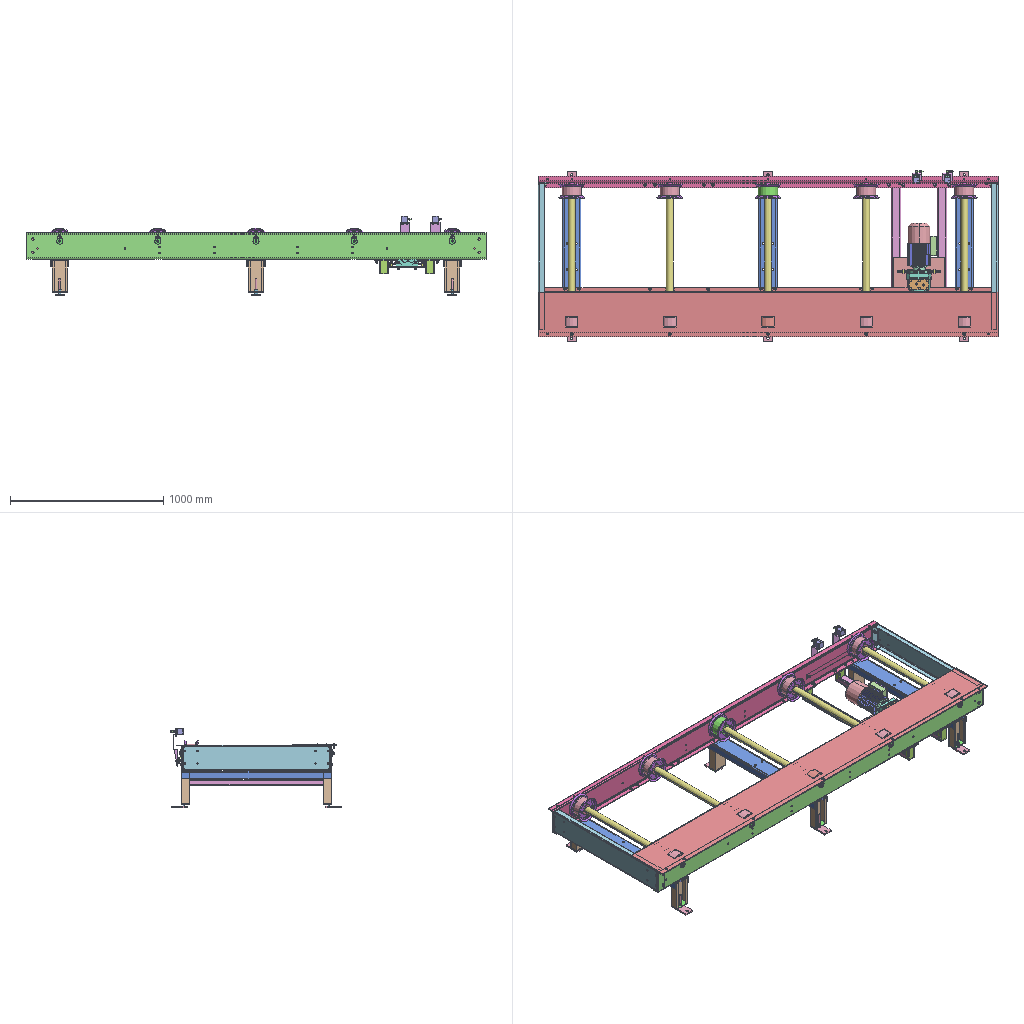Assembly | SolidWorks | 116 different items | 587 placed | box 3000 x 1113 x 520 mm
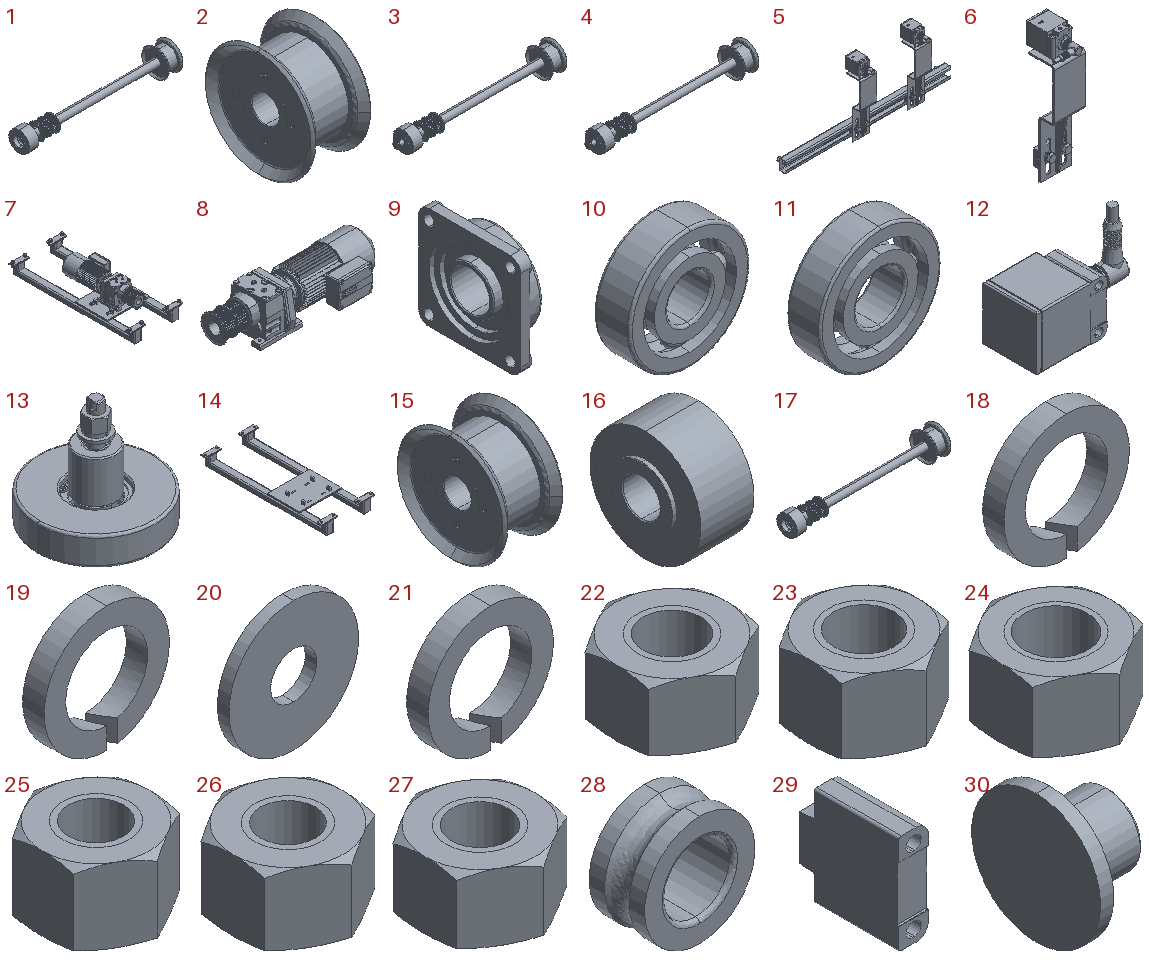Parts list (item | name | quantity | parent item | size | volume | features):
1 | (subassembly) | x1 | in 4 | 930.556 x 169.042 x 169.042 mm | 2373152 mm3 | -
2 | (subassembly) | x1 | in 1 | 91.113 x 169.042 x 169.042 mm | 833344 mm3 | -
3 | (subassembly) | x4 | - | 1011 x 169.042 x 169.042 mm | 2962716 mm3 | -
4 | (subassembly) | x1 | - | 1011 x 169.042 x 169.042 mm | 2962647 mm3 | -
5 | (subassembly) | x2 | - | - | 438614 mm3 | -
6 | (subassembly) | x4 | in 5 | 72 x 82 x 247.45 mm | 157229 mm3 | -
7 | (subassembly) | x1 | - | - | 10349735 mm3 | -
8 | (subassembly) | x1 | in 7 | 565.084 x 209.5 x 152.413 mm | 7667621 mm3 | -
9 | (subassembly) | x1 | - | 96.3 x 235 x 235 mm | 1862383 mm3 | -
10 | (subassembly) | x1 | - | 47 x 14 x 47 mm | 14550 mm3 | -
11 | (subassembly) | x10 | in 3, 4 | 62 x 17 x 62 mm | 29213 mm3 | -
12 | (subassembly) | x4 | in 6 | 82 x 40.45 x 62 mm | 85684 mm3 | -
13 | (subassembly) | x1 | - | 105 x 105 x 95 mm | 244996 mm3 | -
14 | (subassembly) | x1 | in 7 | 425 x 976 x 95 mm | 2540191 mm3 | -
15 | (subassembly) | x4 | in 17 | 91.113 x 169.042 x 169.042 mm | 833344 mm3 | -
16 | (subassembly) | x4 | in 17 | 70 x 125 x 125 mm | 635681 mm3 | -
17 | (subassembly) | x4 | in 3 | 930.556 x 169.042 x 169.042 mm | 2373220 mm3 | -
18 | - | x8 | in 6 | 7.7 x 1.3 x 7.7 mm | 32.877 mm3 | features BaseBody 1
19 | - | x5 | - | 9.3 x 1.6 x 9.3 mm | 59.871 mm3 | features BaseBody 1
20 | - | x7 | - | 18 x 1.6 x 18 mm | 355.679 mm3 | features BaseBody 1
21 | - | x30 | in 3, 4, 5, 6, 7 | 12.3 x 2.1 x 12.3 mm | 136.667 mm3 | features BaseBody 1
22 | - | x20 | in 7 | - | - | features BaseBody 1, RefSurface 1
23 | - | x1 | - | - | - | features BaseBody 1, RefSurface 1
24 | - | x1 | - | - | - | features BaseBody 1, RefSurface 1
25 | - | x8 | in 6 | - | - | features BaseBody 1, RefSurface 1
26 | - | x5 | - | - | - | features BaseBody 1, RefSurface 1
27 | - | x8 | in 5, 7 | - | - | features BaseBody 1, RefSurface 1
28 | - | x1 | - | 27.8 x 14 x 27.8 mm | 4698 mm3 | features BaseBody 1
29 | - | x4 | in 12 | 12 x 40 x 40 mm | 13903 mm3 | features BaseBody 1
30 | - | x4 | in 12 | 12.5 x 22.1 x 22.1 mm | 1625 mm3 | features BaseBody 1
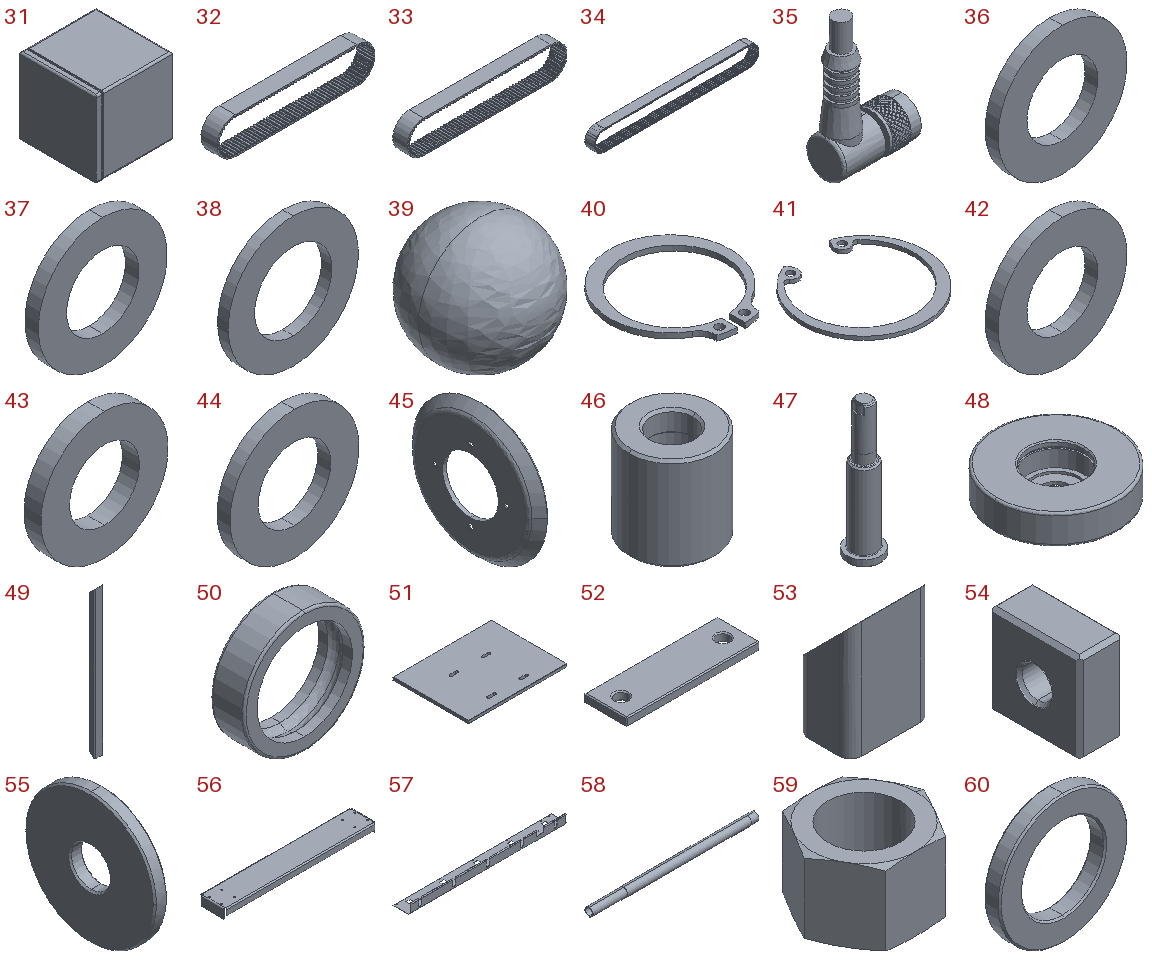31 | - | x4 | in 12 | 40 x 40.45 x 40 mm | 63851 mm3 | features BaseBody 1
32 | - | x1 | - | 394.448 x 40 x 90.448 mm | 157059 mm3 | features BaseBody 1
33 | - | x1 | - | 442.448 x 40 x 90.448 mm | 174219 mm3 | features BaseBody 1
34 | - | x3 | - | 730.448 x 40 x 90.448 mm | 277178 mm3 | features BaseBody 1
35 | - | x4 | in 12 | 29 x 14.5 x 49.25 mm | 6305 mm3 | features BaseBody 1
36 | - | x35 | in 7, 8 | 20 x 2 x 20 mm | 438.252 mm3 | features BaseBody 1
37 | - | x1 | - | 24 x 2.5 x 24 mm | 773.126 mm3 | features BaseBody 1
38 | - | x1 | - | 37 x 3 x 37 mm | 2085 mm3 | features BaseBody 1
39 | - | x1 | - | 7.5 x 7.5 x 7.5 mm | 220.888 mm3 | features BaseBody 1
40 | - | x10 | in 3, 4 | 28.327 x 30.963 x 1.2 mm | 236.217 mm3 | features BaseBody 1
41 | - | x1 | - | 49.5 x 47.444 x 1.5 mm | 686.151 mm3 | features BaseBody 1
42 | - | x8 | in 6 | 10 x 1 x 10 mm | 54.782 mm3 | features BaseBody 1
43 | - | x5 | - | 12 x 1.6 x 12 mm | 126.217 mm3 | features BaseBody 1
44 | - | x20 | in 5, 6, 7 | 16 x 1.6 x 16 mm | 219.911 mm3 | features BaseBody 1
45 | - | x10 | in 2, 15 | 15.556 x 169.042 x 169.042 mm | 97536 mm3 | features BaseBody 1
46 | - | x1 | - | 35 x 35 x 41 mm | 28098 mm3 | features BaseBody 1
47 | - | x1 | - | - | - | features BaseBody 1, RefSurface 1
48 | - | x1 | - | 105 x 105 x 25 mm | 176949 mm3 | features BaseBody 1
49 | - | x2 | in 14 | 60 x 40 x 976 mm | 650329 mm3 | features BaseBody 1
50 | - | x10 | in 11 | 62 x 17 x 62 mm | 17853 mm3 | features BaseBody 1
51 | - | x1 | in 14 | 340 x 260 x 10 mm | 873041 mm3 | features BaseBody 1
52 | - | x4 | in 14 | 125 x 40 x 8 mm | 37771 mm3 | features BaseBody 1
53 | - | x4 | in 14 | 60 x 40 x 87 mm | 46551 mm3 | features BaseBody 1
54 | - | x4 | in 14 | - | - | features BaseBody 1, RefSurface 1
55 | - | x1 | in 8 | 4 x 40 x 40 mm | 4533 mm3 | features BaseBody 1
56 | - | x2 | - | 966 x 165 x 60 mm | 947082 mm3 | features BaseBody 1
57 | - | x1 | - | 3000 x 321 x 172 mm | 2714795 mm3 | features BaseBody 1
58 | - | x5 | in 1, 17 | 860 x 45 x 45 mm | 542272 mm3 | features BaseBody 1
59 | - | x12 | - | 19.85 x 17.191 x 12.2 mm | 1737 mm3 | features Cut 2, Chamfer 1, Extrusion 1
60 | - | x10 | in 3, 4 | 40 x 5 x 40 mm | 3678 mm3 | features BaseBody 1
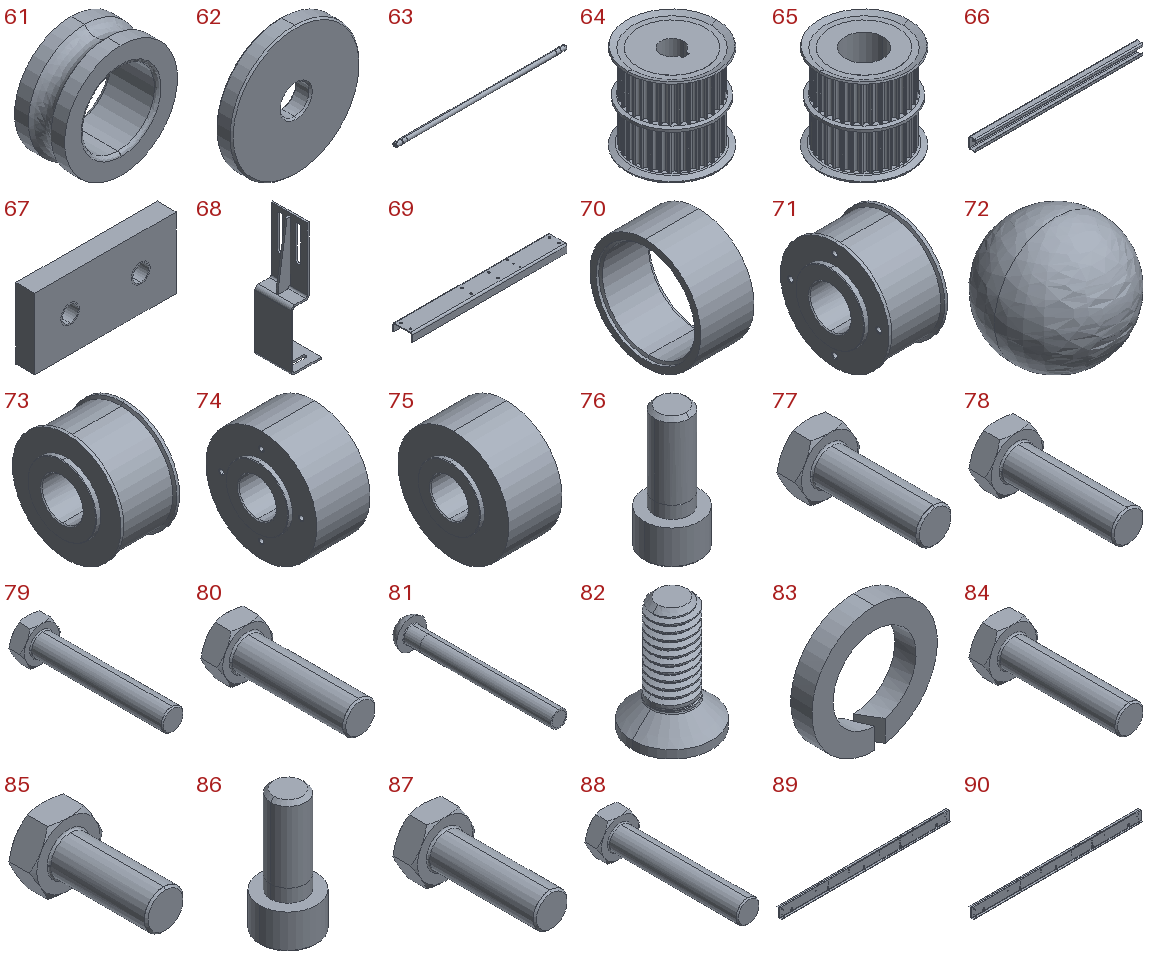61 | - | x10 | in 11 | 38.32 x 17 x 38.32 mm | 9957 mm3 | features BaseBody 1
62 | - | x10 | in 3, 4 | 40 x 5 x 40 mm | 5927 mm3 | features BaseBody 1
63 | - | x5 | in 3, 4 | - | - | features RefSurface 2, BaseBody 1
64 | - | x1 | in 8 | 100.208 x 100.208 x 97.168 mm | 413312 mm3 | features BaseBody 1
65 | - | x5 | in 1, 17 | 100.208 x 100.208 x 97.168 mm | 368257 mm3 | features BaseBody 1
66 | - | x2 | in 5 | 600 x 25 x 40 mm | 115965 mm3 | features BaseBody 1
67 | - | x4 | in 6 | - | - | features RefSurface 2, BaseBody 1
68 | - | x4 | in 6 | 50 x 60 x 207 mm | 49322 mm3 | features BaseBody 1
69 | - | x3 | - | 976 x 120 x 50 mm | 988281 mm3 | features BaseBody 1
70 | - | x8 | in 15, 16 | 60 x 125 x 125 mm | 209654 mm3 | features BaseBody 1
71 | - | x4 | in 15 | - | - | features RefSurface 8, BaseBody 1
72 | - | x40 | in 11 | - | 350.762 mm3 | features BaseBody 1
73 | - | x4 | in 16 | 70 x 111 x 111 mm | 426027 mm3 | features BaseBody 1
74 | - | x1 | in 2 | - | - | features RefSurface 8, BaseBody 1
75 | - | x1 | in 1 | 70 x 125 x 125 mm | 635681 mm3 | features BaseBody 1
76 | - | x1 | in 8 | - | - | features BaseBody 1, RefSurface 1
77 | - | x8 | - | - | - | features BaseBody 1, RefSurface 1
78 | - | x8 | in 7 | - | - | features BaseBody 1, RefSurface 1
79 | - | x4 | in 7 | - | - | features BaseBody 1, RefSurface 1
80 | - | x1 | - | - | - | features BaseBody 1, RefSurface 1
81 | - | x8 | in 6 | - | - | features BaseBody 1, RefSurface 1
82 | - | x40 | in 2, 15 | 11.34 x 11.34 x 16 mm | 524.212 mm3 | features BaseBody 1
83 | - | x35 | in 7, 8 | 15.4 x 2.6 x 15.4 mm | 263.016 mm3 | features BaseBody 1
84 | - | x5 | - | - | - | features BaseBody 1, RefSurface 1
85 | - | x8 | in 6 | - | - | features BaseBody 1, RefSurface 1
86 | - | x4 | in 5 | - | - | features BaseBody 1, RefSurface 1
87 | - | x10 | in 3, 4 | - | - | features BaseBody 1, RefSurface 1
88 | - | x4 | in 7 | - | - | features BaseBody 1, RefSurface 1
89 | - | x1 | - | 3000 x 75 x 170 mm | 3462019 mm3 | features BaseBody 1
90 | - | x1 | - | 3000 x 75 x 170 mm | 3462019 mm3 | features BaseBody 1
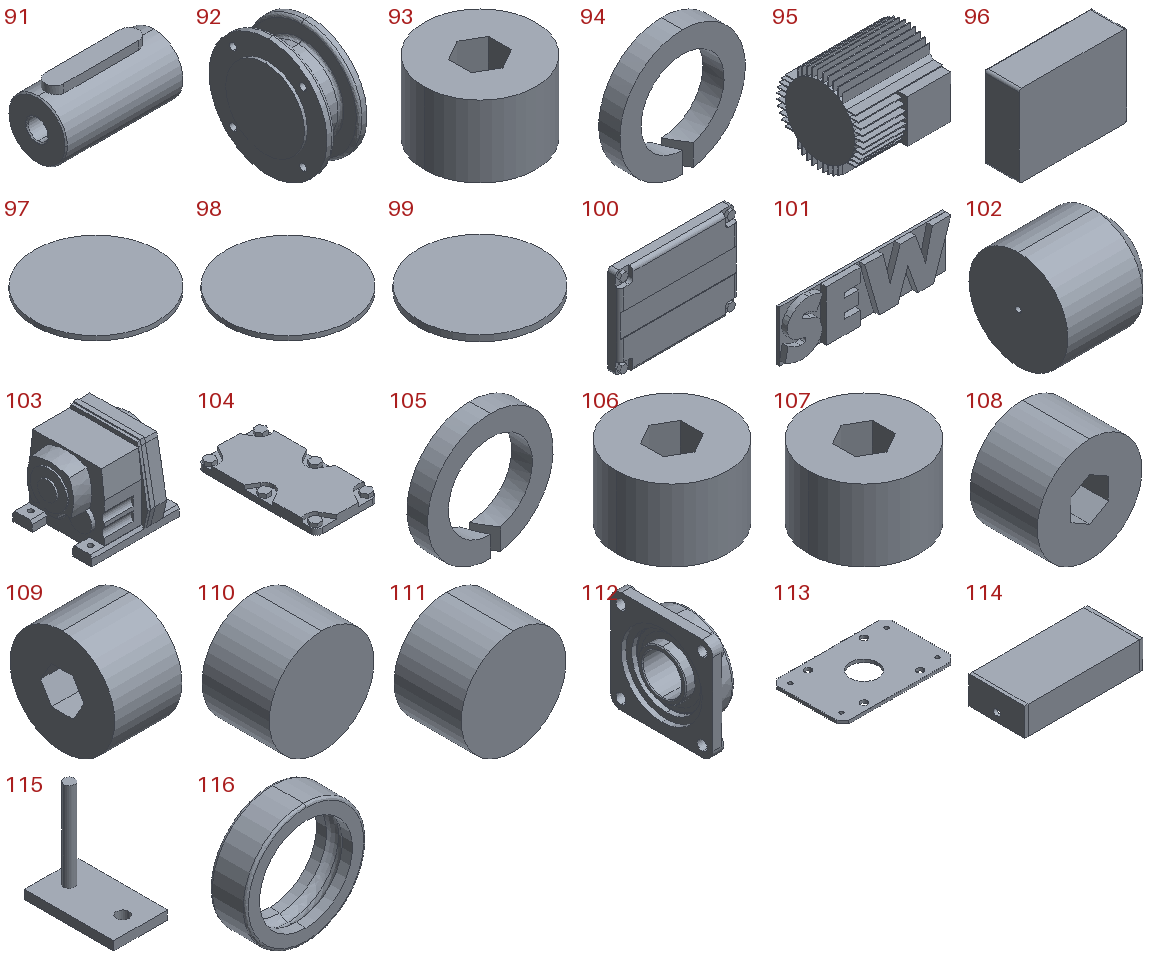91 | - | x1 | in 8 | - | - | features BaseBody 1, RefSurface 1
92 | - | x1 | in 8 | 45 x 120 x 120 mm | 320577 mm3 | features BaseBody 1
93 | - | x1 | in 8 | 14 x 14 x 9 mm | 1299 mm3 | features BaseBody 1
94 | - | x1 | - | 18.4 x 3.1 x 18.4 mm | 446.968 mm3 | features BaseBody 1
95 | - | x1 | in 8 | 146 x 146.326 x 144.651 mm | 1760693 mm3 | features BaseBody 1
96 | - | x1 | in 8 | 125 x 40 x 95 mm | 474597 mm3 | features BaseBody 1
97 | - | x1 | in 8 | 28 x 28 x 4.981 mm | 1761 mm3 | features BaseBody 1
98 | - | x1 | in 8 | 28 x 28 x 4.981 mm | 1761 mm3 | features BaseBody 1
99 | - | x1 | in 8 | 20 x 20 x 3.972 mm | 728.686 mm3 | features BaseBody 1
100 | - | x1 | in 8 | 127 x 13 x 97 mm | 152742 mm3 | features BaseBody 1
101 | - | x1 | in 8 | 58.086 x 3 x 18.091 mm | 2435 mm3 | features BaseBody 1
102 | - | x1 | in 8 | 131 x 145 x 145 mm | 2065871 mm3 | features BaseBody 1
103 | - | x1 | in 8 | 170 x 161 x 147 mm | 2353426 mm3 | features BaseBody 1
104 | - | x1 | in 8 | 66 x 126 x 10 mm | 78056 mm3 | features BaseBody 1
105 | - | x1 | - | 30.2 x 5 x 30.2 mm | 1916 mm3 | features BaseBody 1
106 | - | x1 | in 8 | 14 x 14 x 9 mm | 1299 mm3 | features BaseBody 1
107 | - | x1 | in 8 | 14 x 14 x 9 mm | 1299 mm3 | features BaseBody 1
108 | - | x1 | in 8 | 14 x 9 x 14 mm | 1299 mm3 | features BaseBody 1
109 | - | x1 | in 8 | 9 x 14 x 14 mm | 1299 mm3 | features BaseBody 1
110 | - | x1 | in 8 | 14 x 9 x 14 mm | 1299 mm3 | features BaseBody 1
111 | - | x1 | in 8 | 14 x 9 x 14 mm | 1299 mm3 | features BaseBody 1
112 | - | x1 | - | 96.3 x 235 x 235 mm | 1862383 mm3 | features BaseBody 1
113 | - | x1 | - | 380 x 240 x 10 mm | 816381 mm3 | features BaseBody 1
114 | - | x6 | - | 212 x 100 x 50 mm | 126521 mm3 | features ICE 3, 3DProfileFeature 1, WeldMemberFeat 1, WeldmentFeature 1
115 | - | x6 | - | 60 x 100 x 110 mm | 69770 mm3 | features Extrusion 1, ICE 1
116 | - | x1 | - | 47 x 14 x 47 mm | 8969 mm3 | features BaseBody 1
Mates (type | each side: item.copy, entity, surface, feature):
Coincident | 90.1 edge | 69.1 face plane Input 1
Width | 90.1 face plane Input 1 | 89.1 face plane Input 1 | 69.1 face plane Input 1 | 69.1 face plane Input 1
DistanceDim | 69.1 face plane Input 1 | 56.1 face plane Input 1
Coincident | 89.1 face plane Input 1 | 69.2 face plane Input 1
Coincident | 89.1 face plane Input 1 | 69.3 face plane Input 1 | 2 times
DistanceDim | 69.2 face plane Input 1 | 56.2 face plane Input 1
Coincident | 89.1 face plane Input 1 | 69.1 face plane Input 1
Width | 69.3 face plane Input 1 | 69.3 face plane Input 1 | 69.2 face plane Input 1 | 69.1 face plane Input 1
Coincident | 69.2 face plane Input 1 | 114.1 face plane Boss-Extrude1 | 2 times
Width | 114.1 face plane C-channel C80X40X15X1.5(1) | 114.1 face plane C-channel C80X40X15X1.5(1) | 69.2 face plane Input 1 | 69.2 face plane Input 1
Coincident | 69.2 face plane Input 1 | 114.2 face plane Boss-Extrude1 | 2 times
Width | 114.2 face plane C-channel C80X40X15X1.5(1) | 114.2 face plane C-channel C80X40X15X1.5(1) | 69.2 face plane Input 1 | 69.2 face plane Input 1
Concentric | 114.2 face cylinder Cut-Extrude1 | 115.1 face cylinder Boss-Extrude2
Parallel | 114.2 face plane C-channel C80X40X15X1.5(1) | 115.1 face plane Boss-Extrude1
Concentric | 114.1 face cylinder Cut-Extrude1 | 115.2 face cylinder Boss-Extrude2
Parallel | 114.1 face plane C-channel C80X40X15X1.5(1) | 115.2 face plane Boss-Extrude1
Concentric | 115.1 face cylinder Boss-Extrude2 | 59.1 face cylinder Base-Extrude
Coincident | 114.2 face plane Boss-Extrude2 | 59.2 face plane Base-Extrude
Concentric | 115.1 face cylinder Boss-Extrude2 | 59.2 face cylinder Base-Extrude
Coincident | 114.1 face plane Boss-Extrude2 | 59.3 face plane Base-Extrude
Concentric | 115.2 face cylinder Boss-Extrude2 | 59.3 face cylinder Base-Extrude
Coincident | 114.1 face plane Boss-Extrude2 | 59.4 face plane Base-Extrude
Concentric | 115.2 face cylinder Boss-Extrude2 | 59.4 face cylinder Base-Extrude
Coincident | 90.1 face plane Input 1 | 69.2 face plane Input 1
Coincident | 115.2 face plane Boss-Extrude1 | 59.4 face plane Base-Extrude
Coincident | 114.2 face plane Boss-Extrude2 | 59.1 face plane Base-Extrude
Coincident | 115.1 face plane Boss-Extrude1 | 59.2 face plane Base-Extrude